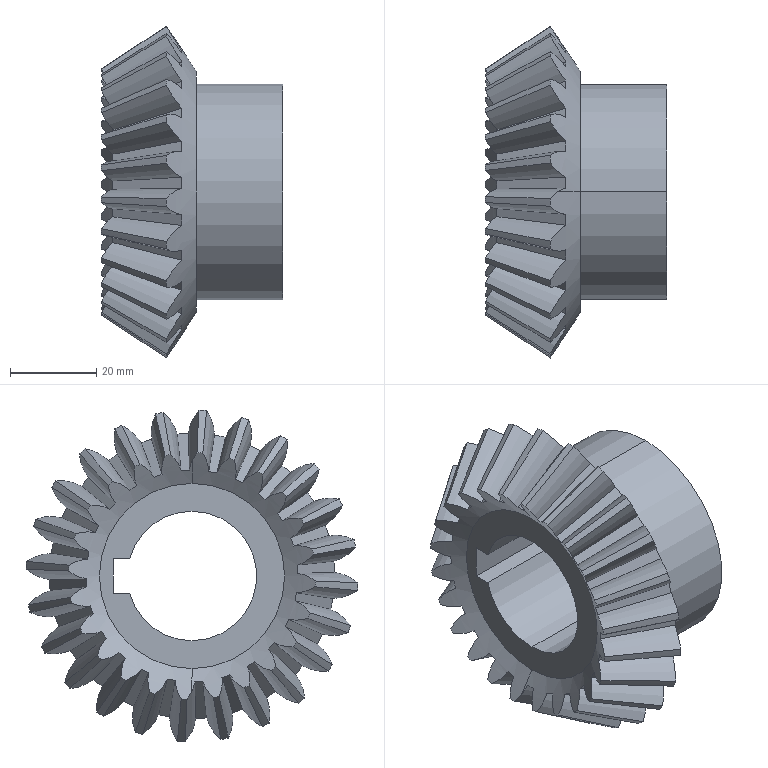Part | STEP file | BEVEL_GEAR_24V11 | 1 solid | 111 faces | box 41.964 x 76.945 x 76.945 mm | volume 70048 mm3 | spline 72 | cone 28 | plane 6 | cylinder 5 | commonest cylinder face diameters 30 x3 50 x2